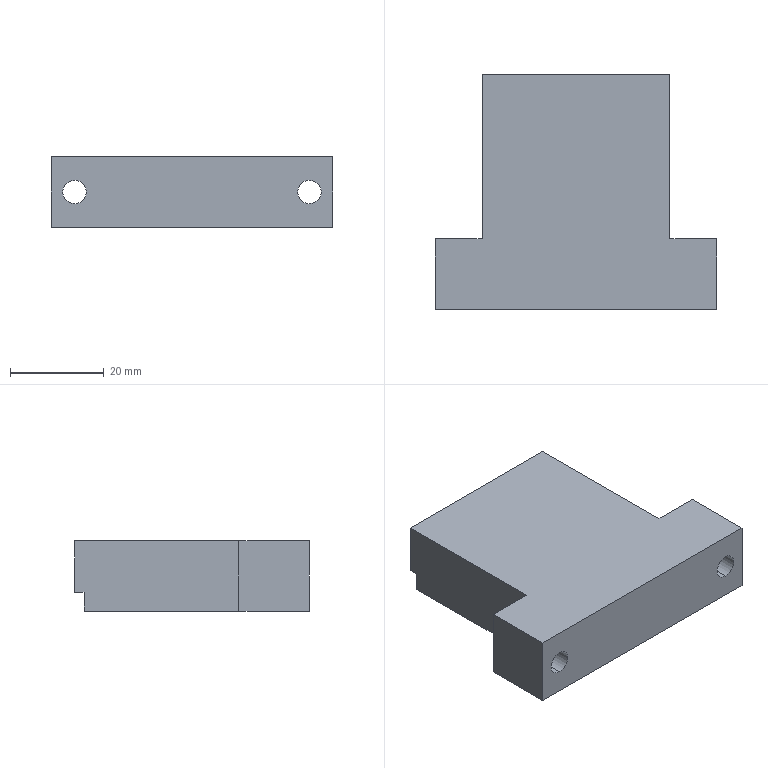Part | STEP file | track spacer block 2 | 1 solid | 28 faces | box 60 x 50 x 15 mm | volume 33477 mm3 | plane 12 | cylinder 10 | cone 6 | commonest cylinder face diameters 2.5 x6 5 x4